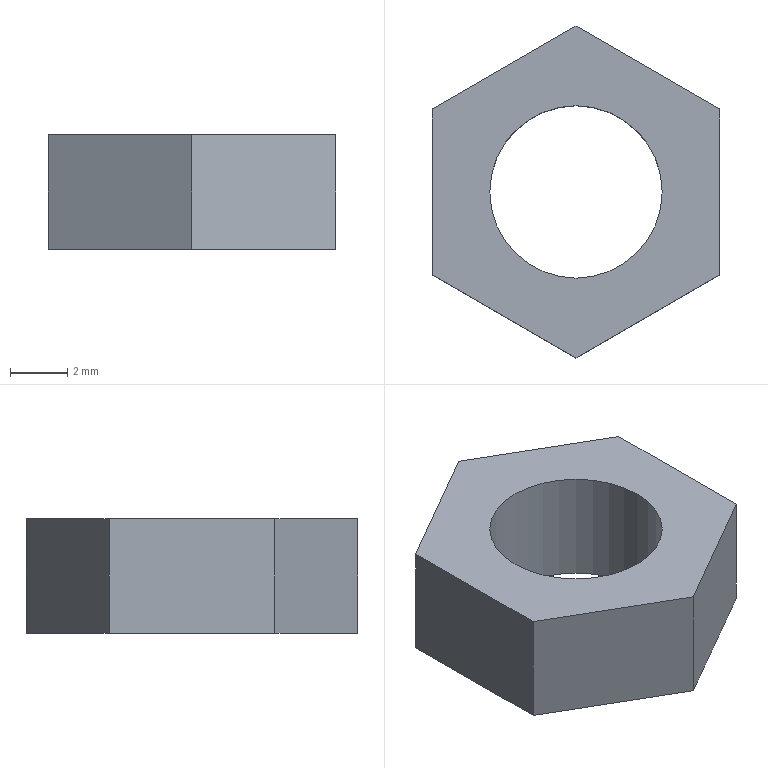Part | STEP file | M6 nut | 1 solid | 10 faces | box 10 x 11.547 x 4 mm | volume 233.313 mm3 | plane 8 | cylinder 2 | commonest cylinder face diameters 6 x2
STEP:
#1=CARTESIAN_POINT('',(0.,0.,0.));
#2=DIRECTION('',(0.,0.,1.));
#3=DIRECTION('',(1.,0.,0.));
#4=AXIS2_PLACEMENT_3D('',#1,#2,#3);
#5=CARTESIAN_POINT('',(-3.,0.,4.));
#6=VERTEX_POINT('',#5);
#7=CARTESIAN_POINT('',(-3.,0.,0.));
#8=VERTEX_POINT('',#7);
#9=CARTESIAN_POINT('',(-3.,0.,4.));
#10=DIRECTION('',(0.,0.,-1.));
#11=VECTOR('',#10,1.);
#12=LINE('',#9,#11);
#13=CARTESIAN_POINT('',(0.,0.,4.));
#14=DIRECTION('',(0.,0.,-1.));
#15=DIRECTION('',(-1.,0.,0.));
#16=AXIS2_PLACEMENT_3D('',#13,#14,#15);
#17=CYLINDRICAL_SURFACE('',#16,3.);
#18=CARTESIAN_POINT('',(6.283,0.));
#19=DIRECTION('',(0.,1.));
#20=VECTOR('',#19,1.);
#21=LINE('',#18,#20);
#22=(GEOMETRIC_REPRESENTATION_CONTEXT(2)PARAMETRIC_REPRESENTATION_CONTEXT()REPRESENTATION_CONTEXT('',''));
#23=DEFINITIONAL_REPRESENTATION('',(#21),#22);
#24=PCURVE('',#17,#23);
#25=CARTESIAN_POINT('',(0.,0.,4.));
#26=DIRECTION('',(0.,0.,-1.));
#27=DIRECTION('',(-1.,0.,0.));
#28=AXIS2_PLACEMENT_3D('',#25,#26,#27);
#29=CYLINDRICAL_SURFACE('',#28,3.);
#30=CARTESIAN_POINT('',(0.,0.));
#31=DIRECTION('',(0.,1.));
#32=VECTOR('',#31,1.);
#33=LINE('',#30,#32);
#34=(GEOMETRIC_REPRESENTATION_CONTEXT(2)PARAMETRIC_REPRESENTATION_CONTEXT()REPRESENTATION_CONTEXT('',''));
#35=DEFINITIONAL_REPRESENTATION('',(#33),#34);
#36=PCURVE('',#29,#35);
#37=SURFACE_CURVE('',#12,(#24,#36),.PCURVE_S1.);
#38=EDGE_CURVE('',#6,#8,#37,.T.);
#39=ORIENTED_EDGE('',*,*,#38,.T.);
#40=CARTESIAN_POINT('',(3.,0.,0.));
#41=VERTEX_POINT('',#40);
#42=CARTESIAN_POINT('',(0.,0.,0.));
#43=DIRECTION('',(0.,0.,1.));
#44=DIRECTION('',(1.,0.,0.));
#45=AXIS2_PLACEMENT_3D('',#42,#43,#44);
#46=CIRCLE('',#45,3.);
#47=CARTESIAN_POINT('',(9.425,4.));
#48=DIRECTION('',(-1.,0.));
#49=VECTOR('',#48,1.);
#50=LINE('',#47,#49);
#51=(GEOMETRIC_REPRESENTATION_CONTEXT(2)PARAMETRIC_REPRESENTATION_CONTEXT()REPRESENTATION_CONTEXT('',''));
#52=DEFINITIONAL_REPRESENTATION('',(#50),#51);
#53=PCURVE('',#17,#52);
#54=CARTESIAN_POINT('',(0.,0.,0.));
#55=DIRECTION('',(0.,0.,1.));
#56=DIRECTION('',(1.,0.,0.));
#57=AXIS2_PLACEMENT_3D('',#54,#55,#56);
#58=PLANE('',#57);
#59=CARTESIAN_POINT('',(0.,0.));
#60=DIRECTION('',(1.,0.));
#61=AXIS2_PLACEMENT_2D('',#59,#60);
#62=CIRCLE('',#61,3.);
#63=(GEOMETRIC_REPRESENTATION_CONTEXT(2)PARAMETRIC_REPRESENTATION_CONTEXT()REPRESENTATION_CONTEXT('',''));
#64=DEFINITIONAL_REPRESENTATION('',(#62),#63);
#65=PCURVE('',#58,#64);
#66=SURFACE_CURVE('',#46,(#53,#65),.PCURVE_S1.);
#67=EDGE_CURVE('',#8,#41,#66,.T.);
#68=ORIENTED_EDGE('',*,*,#67,.T.);
#69=CARTESIAN_POINT('',(3.,0.,4.));
#70=VERTEX_POINT('',#69);
#71=CARTESIAN_POINT('',(3.,0.,4.));
#72=DIRECTION('',(0.,0.,-1.));
#73=VECTOR('',#72,1.);
#74=LINE('',#71,#73);
#75=CARTESIAN_POINT('',(3.142,0.));
#76=DIRECTION('',(0.,1.));
#77=VECTOR('',#76,1.);
#78=LINE('',#75,#77);
#79=(GEOMETRIC_REPRESENTATION_CONTEXT(2)PARAMETRIC_REPRESENTATION_CONTEXT()REPRESENTATION_CONTEXT('',''));
#80=DEFINITIONAL_REPRESENTATION('',(#78),#79);
#81=PCURVE('',#17,#80);
#82=CARTESIAN_POINT('',(3.142,0.));
#83=DIRECTION('',(0.,1.));
#84=VECTOR('',#83,1.);
#85=LINE('',#82,#84);
#86=(GEOMETRIC_REPRESENTATION_CONTEXT(2)PARAMETRIC_REPRESENTATION_CONTEXT()REPRESENTATION_CONTEXT('',''));
#87=DEFINITIONAL_REPRESENTATION('',(#85),#86);
#88=PCURVE('',#29,#87);
#89=SURFACE_CURVE('',#74,(#81,#88),.PCURVE_S1.);
#90=EDGE_CURVE('',#70,#41,#89,.T.);
#91=ORIENTED_EDGE('',*,*,#90,.F.);
#92=CARTESIAN_POINT('',(0.,0.,4.));
#93=DIRECTION('',(0.,0.,1.));
#94=DIRECTION('',(1.,0.,0.));
#95=AXIS2_PLACEMENT_3D('',#92,#93,#94);
#96=CIRCLE('',#95,3.);
#97=CARTESIAN_POINT('',(9.425,0.));
#98=DIRECTION('',(-1.,0.));
#99=VECTOR('',#98,1.);
#100=LINE('',#97,#99);
#101=(GEOMETRIC_REPRESENTATION_CONTEXT(2)PARAMETRIC_REPRESENTATION_CONTEXT()REPRESENTATION_CONTEXT('',''));
#102=DEFINITIONAL_REPRESENTATION('',(#100),#101);
#103=PCURVE('',#17,#102);
#104=CARTESIAN_POINT('',(0.,0.,4.));
#105=DIRECTION('',(0.,0.,1.));
#106=DIRECTION('',(1.,0.,0.));
#107=AXIS2_PLACEMENT_3D('',#104,#105,#106);
#108=PLANE('',#107);
#109=CARTESIAN_POINT('',(0.,0.));
#110=DIRECTION('',(1.,0.));
#111=AXIS2_PLACEMENT_2D('',#109,#110);
#112=CIRCLE('',#111,3.);
#113=(GEOMETRIC_REPRESENTATION_CONTEXT(2)PARAMETRIC_REPRESENTATION_CONTEXT()REPRESENTATION_CONTEXT('',''));
#114=DEFINITIONAL_REPRESENTATION('',(#112),#113);
#115=PCURVE('',#108,#114);
#116=SURFACE_CURVE('',#96,(#103,#115),.PCURVE_S1.);
#117=EDGE_CURVE('',#6,#70,#116,.T.);
#118=ORIENTED_EDGE('',*,*,#117,.F.);
#119=EDGE_LOOP('',(#39,#68,#91,#118));
#120=FACE_BOUND('',#119,.F.);
#121=ADVANCED_FACE('',(#120),#17,.F.);
#122=CARTESIAN_POINT('',(-5.,2.887,4.));
#123=VERTEX_POINT('',#122);
#124=CARTESIAN_POINT('',(-5.,-2.887,4.));
#125=VERTEX_POINT('',#124);
#126=CARTESIAN_POINT('',(-5.,2.887,4.));
#127=DIRECTION('',(0.,-1.,0.));
#128=VECTOR('',#127,1.);
#129=LINE('',#126,#128);
#130=CARTESIAN_POINT('',(-5.,2.887));
#131=DIRECTION('',(0.,-1.));
#132=VECTOR('',#131,1.);
#133=LINE('',#130,#132);
#134=(GEOMETRIC_REPRESENTATION_CONTEXT(2)PARAMETRIC_REPRESENTATION_CONTEXT()REPRESENTATION_CONTEXT('',''));
#135=DEFINITIONAL_REPRESENTATION('',(#133),#134);
#136=PCURVE('',#108,#135);
#137=CARTESIAN_POINT('',(-5.,2.887,4.));
#138=DIRECTION('',(1.,0.,0.));
#139=DIRECTION('',(0.,1.,0.));
#140=AXIS2_PLACEMENT_3D('',#137,#138,#139);
#141=PLANE('',#140);
#142=CARTESIAN_POINT('',(0.,0.));
#143=DIRECTION('',(-1.,0.));
#144=VECTOR('',#143,1.);
#145=LINE('',#142,#144);
#146=(GEOMETRIC_REPRESENTATION_CONTEXT(2)PARAMETRIC_REPRESENTATION_CONTEXT()REPRESENTATION_CONTEXT('',''));
#147=DEFINITIONAL_REPRESENTATION('',(#145),#146);
#148=PCURVE('',#141,#147);
#149=SURFACE_CURVE('',#129,(#136,#148),.PCURVE_S1.);
#150=EDGE_CURVE('',#123,#125,#149,.T.);
#151=ORIENTED_EDGE('',*,*,#150,.T.);
#152=CARTESIAN_POINT('',(0.,-5.774,4.));
#153=VERTEX_POINT('',#152);
#154=CARTESIAN_POINT('',(-5.,-2.887,4.));
#155=DIRECTION('',(0.866,-0.5,0.));
#156=VECTOR('',#155,1.);
#157=LINE('',#154,#156);
#158=CARTESIAN_POINT('',(-5.,-2.887));
#159=DIRECTION('',(0.866,-0.5));
#160=VECTOR('',#159,1.);
#161=LINE('',#158,#160);
#162=(GEOMETRIC_REPRESENTATION_CONTEXT(2)PARAMETRIC_REPRESENTATION_CONTEXT()REPRESENTATION_CONTEXT('',''));
#163=DEFINITIONAL_REPRESENTATION('',(#161),#162);
#164=PCURVE('',#108,#163);
#165=CARTESIAN_POINT('',(-5.,-2.887,4.));
#166=DIRECTION('',(0.5,0.866,0.));
#167=DIRECTION('',(-0.866,0.5,0.));
#168=AXIS2_PLACEMENT_3D('',#165,#166,#167);
#169=PLANE('',#168);
#170=CARTESIAN_POINT('',(0.,0.));
#171=DIRECTION('',(-1.,0.));
#172=VECTOR('',#171,1.);
#173=LINE('',#170,#172);
#174=(GEOMETRIC_REPRESENTATION_CONTEXT(2)PARAMETRIC_REPRESENTATION_CONTEXT()REPRESENTATION_CONTEXT('',''));
#175=DEFINITIONAL_REPRESENTATION('',(#173),#174);
#176=PCURVE('',#169,#175);
#177=SURFACE_CURVE('',#157,(#164,#176),.PCURVE_S1.);
#178=EDGE_CURVE('',#125,#153,#177,.T.);
#179=ORIENTED_EDGE('',*,*,#178,.T.);
#180=CARTESIAN_POINT('',(5.,-2.887,4.));
#181=VERTEX_POINT('',#180);
#182=CARTESIAN_POINT('',(0.,-5.774,4.));
#183=DIRECTION('',(0.866,0.5,0.));
#184=VECTOR('',#183,1.);
#185=LINE('',#182,#184);
#186=CARTESIAN_POINT('',(0.,-5.774));
#187=DIRECTION('',(0.866,0.5));
#188=VECTOR('',#187,1.);
#189=LINE('',#186,#188);
#190=(GEOMETRIC_REPRESENTATION_CONTEXT(2)PARAMETRIC_REPRESENTATION_CONTEXT()REPRESENTATION_CONTEXT('',''));
#191=DEFINITIONAL_REPRESENTATION('',(#189),#190);
#192=PCURVE('',#108,#191);
#193=CARTESIAN_POINT('',(0.,-5.774,4.));
#194=DIRECTION('',(-0.5,0.866,0.));
#195=DIRECTION('',(-0.866,-0.5,0.));
#196=AXIS2_PLACEMENT_3D('',#193,#194,#195);
#197=PLANE('',#196);
#198=CARTESIAN_POINT('',(0.,0.));
#199=DIRECTION('',(-1.,0.));
#200=VECTOR('',#199,1.);
#201=LINE('',#198,#200);
#202=(GEOMETRIC_REPRESENTATION_CONTEXT(2)PARAMETRIC_REPRESENTATION_CONTEXT()REPRESENTATION_CONTEXT('',''));
#203=DEFINITIONAL_REPRESENTATION('',(#201),#202);
#204=PCURVE('',#197,#203);
#205=SURFACE_CURVE('',#185,(#192,#204),.PCURVE_S1.);
#206=EDGE_CURVE('',#153,#181,#205,.T.);
#207=ORIENTED_EDGE('',*,*,#206,.T.);
#208=CARTESIAN_POINT('',(5.,2.887,4.));
#209=VERTEX_POINT('',#208);
#210=CARTESIAN_POINT('',(5.,-2.887,4.));
#211=DIRECTION('',(0.,1.,0.));
#212=VECTOR('',#211,1.);
#213=LINE('',#210,#212);
#214=CARTESIAN_POINT('',(5.,-2.887));
#215=DIRECTION('',(0.,1.));
#216=VECTOR('',#215,1.);
#217=LINE('',#214,#216);
#218=(GEOMETRIC_REPRESENTATION_CONTEXT(2)PARAMETRIC_REPRESENTATION_CONTEXT()REPRESENTATION_CONTEXT('',''));
#219=DEFINITIONAL_REPRESENTATION('',(#217),#218);
#220=PCURVE('',#108,#219);
#221=CARTESIAN_POINT('',(5.,-2.887,4.));
#222=DIRECTION('',(-1.,0.,0.));
#223=DIRECTION('',(0.,0.,1.));
#224=AXIS2_PLACEMENT_3D('',#221,#222,#223);
#225=PLANE('',#224);
#226=CARTESIAN_POINT('',(0.,0.));
#227=DIRECTION('',(0.,1.));
#228=VECTOR('',#227,1.);
#229=LINE('',#226,#228);
#230=(GEOMETRIC_REPRESENTATION_CONTEXT(2)PARAMETRIC_REPRESENTATION_CONTEXT()REPRESENTATION_CONTEXT('',''));
#231=DEFINITIONAL_REPRESENTATION('',(#229),#230);
#232=PCURVE('',#225,#231);
#233=SURFACE_CURVE('',#213,(#220,#232),.PCURVE_S1.);
#234=EDGE_CURVE('',#181,#209,#233,.T.);
#235=ORIENTED_EDGE('',*,*,#234,.T.);
#236=CARTESIAN_POINT('',(0.,5.774,4.));
#237=VERTEX_POINT('',#236);
#238=CARTESIAN_POINT('',(5.,2.887,4.));
#239=DIRECTION('',(-0.866,0.5,0.));
#240=VECTOR('',#239,1.);
#241=LINE('',#238,#240);
#242=CARTESIAN_POINT('',(5.,2.887));
#243=DIRECTION('',(-0.866,0.5));
#244=VECTOR('',#243,1.);
#245=LINE('',#242,#244);
#246=(GEOMETRIC_REPRESENTATION_CONTEXT(2)PARAMETRIC_REPRESENTATION_CONTEXT()REPRESENTATION_CONTEXT('',''));
#247=DEFINITIONAL_REPRESENTATION('',(#245),#246);
#248=PCURVE('',#108,#247);
#249=CARTESIAN_POINT('',(5.,2.887,4.));
#250=DIRECTION('',(-0.5,-0.866,0.));
#251=DIRECTION('',(0.866,-0.5,0.));
#252=AXIS2_PLACEMENT_3D('',#249,#250,#251);
#253=PLANE('',#252);
#254=CARTESIAN_POINT('',(0.,0.));
#255=DIRECTION('',(-1.,0.));
#256=VECTOR('',#255,1.);
#257=LINE('',#254,#256);
#258=(GEOMETRIC_REPRESENTATION_CONTEXT(2)PARAMETRIC_REPRESENTATION_CONTEXT()REPRESENTATION_CONTEXT('',''));
#259=DEFINITIONAL_REPRESENTATION('',(#257),#258);
#260=PCURVE('',#253,#259);
#261=SURFACE_CURVE('',#241,(#248,#260),.PCURVE_S1.);
#262=EDGE_CURVE('',#209,#237,#261,.T.);
#263=ORIENTED_EDGE('',*,*,#262,.T.);
#264=CARTESIAN_POINT('',(0.,5.774,4.));
#265=DIRECTION('',(-0.866,-0.5,0.));
#266=VECTOR('',#265,1.);
#267=LINE('',#264,#266);
#268=CARTESIAN_POINT('',(0.,5.774));
#269=DIRECTION('',(-0.866,-0.5));
#270=VECTOR('',#269,1.);
#271=LINE('',#268,#270);
#272=(GEOMETRIC_REPRESENTATION_CONTEXT(2)PARAMETRIC_REPRESENTATION_CONTEXT()REPRESENTATION_CONTEXT('',''));
#273=DEFINITIONAL_REPRESENTATION('',(#271),#272);
#274=PCURVE('',#108,#273);
#275=CARTESIAN_POINT('',(0.,5.774,4.));
#276=DIRECTION('',(0.5,-0.866,0.));
#277=DIRECTION('',(0.866,0.5,0.));
#278=AXIS2_PLACEMENT_3D('',#275,#276,#277);
#279=PLANE('',#278);
#280=CARTESIAN_POINT('',(0.,0.));
#281=DIRECTION('',(-1.,0.));
#282=VECTOR('',#281,1.);
#283=LINE('',#280,#282);
#284=(GEOMETRIC_REPRESENTATION_CONTEXT(2)PARAMETRIC_REPRESENTATION_CONTEXT()REPRESENTATION_CONTEXT('',''));
#285=DEFINITIONAL_REPRESENTATION('',(#283),#284);
#286=PCURVE('',#279,#285);
#287=SURFACE_CURVE('',#267,(#274,#286),.PCURVE_S1.);
#288=EDGE_CURVE('',#237,#123,#287,.T.);
#289=ORIENTED_EDGE('',*,*,#288,.T.);
#290=EDGE_LOOP('',(#151,#179,#207,#235,#263,#289));
#291=FACE_BOUND('',#290,.T.);
#292=ORIENTED_EDGE('',*,*,#117,.F.);
#293=CARTESIAN_POINT('',(0.,0.,4.));
#294=DIRECTION('',(0.,0.,1.));
#295=DIRECTION('',(1.,0.,0.));
#296=AXIS2_PLACEMENT_3D('',#293,#294,#295);
#297=CIRCLE('',#296,3.);
#298=CARTESIAN_POINT('',(0.,0.));
#299=DIRECTION('',(1.,0.));
#300=AXIS2_PLACEMENT_2D('',#298,#299);
#301=CIRCLE('',#300,3.);
#302=(GEOMETRIC_REPRESENTATION_CONTEXT(2)PARAMETRIC_REPRESENTATION_CONTEXT()REPRESENTATION_CONTEXT('',''));
#303=DEFINITIONAL_REPRESENTATION('',(#301),#302);
#304=PCURVE('',#108,#303);
#305=CARTESIAN_POINT('',(3.142,0.));
#306=DIRECTION('',(-1.,0.));
#307=VECTOR('',#306,1.);
#308=LINE('',#305,#307);
#309=(GEOMETRIC_REPRESENTATION_CONTEXT(2)PARAMETRIC_REPRESENTATION_CONTEXT()REPRESENTATION_CONTEXT('',''));
#310=DEFINITIONAL_REPRESENTATION('',(#308),#309);
#311=PCURVE('',#29,#310);
#312=SURFACE_CURVE('',#297,(#304,#311),.PCURVE_S1.);
#313=EDGE_CURVE('',#70,#6,#312,.T.);
#314=ORIENTED_EDGE('',*,*,#313,.F.);
#315=EDGE_LOOP('',(#292,#314));
#316=FACE_BOUND('',#315,.T.);
#317=ADVANCED_FACE('',(#291,#316),#108,.T.);
#318=CARTESIAN_POINT('',(-5.,2.887,0.));
#319=VERTEX_POINT('',#318);
#320=CARTESIAN_POINT('',(-5.,-2.887,0.));
#321=VERTEX_POINT('',#320);
#322=CARTESIAN_POINT('',(-5.,2.887,0.));
#323=DIRECTION('',(0.,-1.,0.));
#324=VECTOR('',#323,1.);
#325=LINE('',#322,#324);
#326=CARTESIAN_POINT('',(-5.,2.887));
#327=DIRECTION('',(0.,-1.));
#328=VECTOR('',#327,1.);
#329=LINE('',#326,#328);
#330=(GEOMETRIC_REPRESENTATION_CONTEXT(2)PARAMETRIC_REPRESENTATION_CONTEXT()REPRESENTATION_CONTEXT('',''));
#331=DEFINITIONAL_REPRESENTATION('',(#329),#330);
#332=PCURVE('',#58,#331);
#333=CARTESIAN_POINT('',(0.,-4.));
#334=DIRECTION('',(-1.,0.));
#335=VECTOR('',#334,1.);
#336=LINE('',#333,#335);
#337=(GEOMETRIC_REPRESENTATION_CONTEXT(2)PARAMETRIC_REPRESENTATION_CONTEXT()REPRESENTATION_CONTEXT('',''));
#338=DEFINITIONAL_REPRESENTATION('',(#336),#337);
#339=PCURVE('',#141,#338);
#340=SURFACE_CURVE('',#325,(#332,#339),.PCURVE_S1.);
#341=EDGE_CURVE('',#319,#321,#340,.T.);
#342=ORIENTED_EDGE('',*,*,#341,.F.);
#343=CARTESIAN_POINT('',(0.,5.774,0.));
#344=VERTEX_POINT('',#343);
#345=CARTESIAN_POINT('',(0.,5.774,0.));
#346=DIRECTION('',(-0.866,-0.5,0.));
#347=VECTOR('',#346,1.);
#348=LINE('',#345,#347);
#349=CARTESIAN_POINT('',(0.,5.774));
#350=DIRECTION('',(-0.866,-0.5));
#351=VECTOR('',#350,1.);
#352=LINE('',#349,#351);
#353=(GEOMETRIC_REPRESENTATION_CONTEXT(2)PARAMETRIC_REPRESENTATION_CONTEXT()REPRESENTATION_CONTEXT('',''));
#354=DEFINITIONAL_REPRESENTATION('',(#352),#353);
#355=PCURVE('',#58,#354);
#356=CARTESIAN_POINT('',(0.,-4.));
#357=DIRECTION('',(-1.,0.));
#358=VECTOR('',#357,1.);
#359=LINE('',#356,#358);
#360=(GEOMETRIC_REPRESENTATION_CONTEXT(2)PARAMETRIC_REPRESENTATION_CONTEXT()REPRESENTATION_CONTEXT('',''));
#361=DEFINITIONAL_REPRESENTATION('',(#359),#360);
#362=PCURVE('',#279,#361);
#363=SURFACE_CURVE('',#348,(#355,#362),.PCURVE_S1.);
#364=EDGE_CURVE('',#344,#319,#363,.T.);
#365=ORIENTED_EDGE('',*,*,#364,.F.);
#366=CARTESIAN_POINT('',(5.,2.887,0.));
#367=VERTEX_POINT('',#366);
#368=CARTESIAN_POINT('',(5.,2.887,0.));
#369=DIRECTION('',(-0.866,0.5,0.));
#370=VECTOR('',#369,1.);
#371=LINE('',#368,#370);
#372=CARTESIAN_POINT('',(5.,2.887));
#373=DIRECTION('',(-0.866,0.5));
#374=VECTOR('',#373,1.);
#375=LINE('',#372,#374);
#376=(GEOMETRIC_REPRESENTATION_CONTEXT(2)PARAMETRIC_REPRESENTATION_CONTEXT()REPRESENTATION_CONTEXT('',''));
#377=DEFINITIONAL_REPRESENTATION('',(#375),#376);
#378=PCURVE('',#58,#377);
#379=CARTESIAN_POINT('',(0.,-4.));
#380=DIRECTION('',(-1.,0.));
#381=VECTOR('',#380,1.);
#382=LINE('',#379,#381);
#383=(GEOMETRIC_REPRESENTATION_CONTEXT(2)PARAMETRIC_REPRESENTATION_CONTEXT()REPRESENTATION_CONTEXT('',''));
#384=DEFINITIONAL_REPRESENTATION('',(#382),#383);
#385=PCURVE('',#253,#384);
#386=SURFACE_CURVE('',#371,(#378,#385),.PCURVE_S1.);
#387=EDGE_CURVE('',#367,#344,#386,.T.);
#388=ORIENTED_EDGE('',*,*,#387,.F.);
#389=CARTESIAN_POINT('',(5.,-2.887,0.));
#390=VERTEX_POINT('',#389);
#391=CARTESIAN_POINT('',(5.,-2.887,0.));
#392=DIRECTION('',(0.,1.,0.));
#393=VECTOR('',#392,1.);
#394=LINE('',#391,#393);
#395=CARTESIAN_POINT('',(5.,-2.887));
#396=DIRECTION('',(0.,1.));
#397=VECTOR('',#396,1.);
#398=LINE('',#395,#397);
#399=(GEOMETRIC_REPRESENTATION_CONTEXT(2)PARAMETRIC_REPRESENTATION_CONTEXT()REPRESENTATION_CONTEXT('',''));
#400=DEFINITIONAL_REPRESENTATION('',(#398),#399);
#401=PCURVE('',#58,#400);
#402=CARTESIAN_POINT('',(-4.,0.));
#403=DIRECTION('',(0.,1.));
#404=VECTOR('',#403,1.);
#405=LINE('',#402,#404);
#406=(GEOMETRIC_REPRESENTATION_CONTEXT(2)PARAMETRIC_REPRESENTATION_CONTEXT()REPRESENTATION_CONTEXT('',''));
#407=DEFINITIONAL_REPRESENTATION('',(#405),#406);
#408=PCURVE('',#225,#407);
#409=SURFACE_CURVE('',#394,(#401,#408),.PCURVE_S1.);
#410=EDGE_CURVE('',#390,#367,#409,.T.);
#411=ORIENTED_EDGE('',*,*,#410,.F.);
#412=CARTESIAN_POINT('',(0.,-5.774,0.));
#413=VERTEX_POINT('',#412);
#414=CARTESIAN_POINT('',(0.,-5.774,0.));
#415=DIRECTION('',(0.866,0.5,0.));
#416=VECTOR('',#415,1.);
#417=LINE('',#414,#416);
#418=CARTESIAN_POINT('',(0.,-5.774));
#419=DIRECTION('',(0.866,0.5));
#420=VECTOR('',#419,1.);
#421=LINE('',#418,#420);
#422=(GEOMETRIC_REPRESENTATION_CONTEXT(2)PARAMETRIC_REPRESENTATION_CONTEXT()REPRESENTATION_CONTEXT('',''));
#423=DEFINITIONAL_REPRESENTATION('',(#421),#422);
#424=PCURVE('',#58,#423);
#425=CARTESIAN_POINT('',(0.,-4.));
#426=DIRECTION('',(-1.,0.));
#427=VECTOR('',#426,1.);
#428=LINE('',#425,#427);
#429=(GEOMETRIC_REPRESENTATION_CONTEXT(2)PARAMETRIC_REPRESENTATION_CONTEXT()REPRESENTATION_CONTEXT('',''));
#430=DEFINITIONAL_REPRESENTATION('',(#428),#429);
#431=PCURVE('',#197,#430);
#432=SURFACE_CURVE('',#417,(#424,#431),.PCURVE_S1.);
#433=EDGE_CURVE('',#413,#390,#432,.T.);
#434=ORIENTED_EDGE('',*,*,#433,.F.);
#435=CARTESIAN_POINT('',(-5.,-2.887,0.));
#436=DIRECTION('',(0.866,-0.5,0.));
#437=VECTOR('',#436,1.);
#438=LINE('',#435,#437);
#439=CARTESIAN_POINT('',(-5.,-2.887));
#440=DIRECTION('',(0.866,-0.5));
#441=VECTOR('',#440,1.);
#442=LINE('',#439,#441);
#443=(GEOMETRIC_REPRESENTATION_CONTEXT(2)PARAMETRIC_REPRESENTATION_CONTEXT()REPRESENTATION_CONTEXT('',''));
#444=DEFINITIONAL_REPRESENTATION('',(#442),#443);
#445=PCURVE('',#58,#444);
#446=CARTESIAN_POINT('',(0.,-4.));
#447=DIRECTION('',(-1.,0.));
#448=VECTOR('',#447,1.);
#449=LINE('',#446,#448);
#450=(GEOMETRIC_REPRESENTATION_CONTEXT(2)PARAMETRIC_REPRESENTATION_CONTEXT()REPRESENTATION_CONTEXT('',''));
#451=DEFINITIONAL_REPRESENTATION('',(#449),#450);
#452=PCURVE('',#169,#451);
#453=SURFACE_CURVE('',#438,(#445,#452),.PCURVE_S1.);
#454=EDGE_CURVE('',#321,#413,#453,.T.);
#455=ORIENTED_EDGE('',*,*,#454,.F.);
#456=EDGE_LOOP('',(#342,#365,#388,#411,#434,#455));
#457=FACE_BOUND('',#456,.T.);
#458=ORIENTED_EDGE('',*,*,#67,.T.);
#459=CARTESIAN_POINT('',(0.,0.,0.));
#460=DIRECTION('',(0.,0.,1.));
#461=DIRECTION('',(1.,0.,0.));
#462=AXIS2_PLACEMENT_3D('',#459,#460,#461);
#463=CIRCLE('',#462,3.);
#464=CARTESIAN_POINT('',(0.,0.));
#465=DIRECTION('',(1.,0.));
#466=AXIS2_PLACEMENT_2D('',#464,#465);
#467=CIRCLE('',#466,3.);
#468=(GEOMETRIC_REPRESENTATION_CONTEXT(2)PARAMETRIC_REPRESENTATION_CONTEXT()REPRESENTATION_CONTEXT('',''));
#469=DEFINITIONAL_REPRESENTATION('',(#467),#468);
#470=PCURVE('',#58,#469);
#471=CARTESIAN_POINT('',(3.142,4.));
#472=DIRECTION('',(-1.,0.));
#473=VECTOR('',#472,1.);
#474=LINE('',#471,#473);
#475=(GEOMETRIC_REPRESENTATION_CONTEXT(2)PARAMETRIC_REPRESENTATION_CONTEXT()REPRESENTATION_CONTEXT('',''));
#476=DEFINITIONAL_REPRESENTATION('',(#474),#475);
#477=PCURVE('',#29,#476);
#478=SURFACE_CURVE('',#463,(#470,#477),.PCURVE_S1.);
#479=EDGE_CURVE('',#41,#8,#478,.T.);
#480=ORIENTED_EDGE('',*,*,#479,.T.);
#481=EDGE_LOOP('',(#458,#480));
#482=FACE_BOUND('',#481,.T.);
#483=ADVANCED_FACE('',(#457,#482),#58,.F.);
#484=ORIENTED_EDGE('',*,*,#341,.T.);
#485=CARTESIAN_POINT('',(-5.,-2.887,4.));
#486=DIRECTION('',(0.,0.,-1.));
#487=VECTOR('',#486,1.);
#488=LINE('',#485,#487);
#489=CARTESIAN_POINT('',(-5.774,0.));
#490=DIRECTION('',(0.,-1.));
#491=VECTOR('',#490,1.);
#492=LINE('',#489,#491);
#493=(GEOMETRIC_REPRESENTATION_CONTEXT(2)PARAMETRIC_REPRESENTATION_CONTEXT()REPRESENTATION_CONTEXT('',''));
#494=DEFINITIONAL_REPRESENTATION('',(#492),#493);
#495=PCURVE('',#141,#494);
#496=CARTESIAN_POINT('',(0.,0.));
#497=DIRECTION('',(0.,-1.));
#498=VECTOR('',#497,1.);
#499=LINE('',#496,#498);
#500=(GEOMETRIC_REPRESENTATION_CONTEXT(2)PARAMETRIC_REPRESENTATION_CONTEXT()REPRESENTATION_CONTEXT('',''));
#501=DEFINITIONAL_REPRESENTATION('',(#499),#500);
#502=PCURVE('',#169,#501);
#503=SURFACE_CURVE('',#488,(#495,#502),.PCURVE_S1.);
#504=EDGE_CURVE('',#125,#321,#503,.T.);
#505=ORIENTED_EDGE('',*,*,#504,.F.);
#506=ORIENTED_EDGE('',*,*,#150,.F.);
#507=CARTESIAN_POINT('',(-5.,2.887,4.));
#508=DIRECTION('',(0.,0.,-1.));
#509=VECTOR('',#508,1.);
#510=LINE('',#507,#509);
#511=CARTESIAN_POINT('',(0.,0.));
#512=DIRECTION('',(0.,-1.));
#513=VECTOR('',#512,1.);
#514=LINE('',#511,#513);
#515=(GEOMETRIC_REPRESENTATION_CONTEXT(2)PARAMETRIC_REPRESENTATION_CONTEXT()REPRESENTATION_CONTEXT('',''));
#516=DEFINITIONAL_REPRESENTATION('',(#514),#515);
#517=PCURVE('',#141,#516);
#518=CARTESIAN_POINT('',(-5.774,0.));
#519=DIRECTION('',(0.,-1.));
#520=VECTOR('',#519,1.);
#521=LINE('',#518,#520);
#522=(GEOMETRIC_REPRESENTATION_CONTEXT(2)PARAMETRIC_REPRESENTATION_CONTEXT()REPRESENTATION_CONTEXT('',''));
#523=DEFINITIONAL_REPRESENTATION('',(#521),#522);
#524=PCURVE('',#279,#523);
#525=SURFACE_CURVE('',#510,(#517,#524),.PCURVE_S1.);
#526=EDGE_CURVE('',#123,#319,#525,.T.);
#527=ORIENTED_EDGE('',*,*,#526,.T.);
#528=EDGE_LOOP('',(#484,#505,#506,#527));
#529=FACE_BOUND('',#528,.T.);
#530=ADVANCED_FACE('',(#529),#141,.F.);
#531=ORIENTED_EDGE('',*,*,#454,.T.);
#532=CARTESIAN_POINT('',(0.,-5.774,4.));
#533=DIRECTION('',(0.,0.,-1.));
#534=VECTOR('',#533,1.);
#535=LINE('',#532,#534);
#536=CARTESIAN_POINT('',(-5.774,0.));
#537=DIRECTION('',(0.,-1.));
#538=VECTOR('',#537,1.);
#539=LINE('',#536,#538);
#540=(GEOMETRIC_REPRESENTATION_CONTEXT(2)PARAMETRIC_REPRESENTATION_CONTEXT()REPRESENTATION_CONTEXT('',''));
#541=DEFINITIONAL_REPRESENTATION('',(#539),#540);
#542=PCURVE('',#169,#541);
#543=CARTESIAN_POINT('',(0.,0.));
#544=DIRECTION('',(0.,-1.));
#545=VECTOR('',#544,1.);
#546=LINE('',#543,#545);
#547=(GEOMETRIC_REPRESENTATION_CONTEXT(2)PARAMETRIC_REPRESENTATION_CONTEXT()REPRESENTATION_CONTEXT('',''));
#548=DEFINITIONAL_REPRESENTATION('',(#546),#547);
#549=PCURVE('',#197,#548);
#550=SURFACE_CURVE('',#535,(#542,#549),.PCURVE_S1.);
#551=EDGE_CURVE('',#153,#413,#550,.T.);
#552=ORIENTED_EDGE('',*,*,#551,.F.);
#553=ORIENTED_EDGE('',*,*,#178,.F.);
#554=ORIENTED_EDGE('',*,*,#504,.T.);
#555=EDGE_LOOP('',(#531,#552,#553,#554));
#556=FACE_BOUND('',#555,.T.);
#557=ADVANCED_FACE('',(#556),#169,.F.);
#558=ORIENTED_EDGE('',*,*,#433,.T.);
#559=CARTESIAN_POINT('',(5.,-2.887,4.));
#560=DIRECTION('',(0.,0.,-1.));
#561=VECTOR('',#560,1.);
#562=LINE('',#559,#561);
#563=CARTESIAN_POINT('',(-5.774,0.));
#564=DIRECTION('',(0.,-1.));
#565=VECTOR('',#564,1.);
#566=LINE('',#563,#565);
#567=(GEOMETRIC_REPRESENTATION_CONTEXT(2)PARAMETRIC_REPRESENTATION_CONTEXT()REPRESENTATION_CONTEXT('',''));
#568=DEFINITIONAL_REPRESENTATION('',(#566),#567);
#569=PCURVE('',#197,#568);
#570=CARTESIAN_POINT('',(0.,0.));
#571=DIRECTION('',(-1.,0.));
#572=VECTOR('',#571,1.);
#573=LINE('',#570,#572);
#574=(GEOMETRIC_REPRESENTATION_CONTEXT(2)PARAMETRIC_REPRESENTATION_CONTEXT()REPRESENTATION_CONTEXT('',''));
#575=DEFINITIONAL_REPRESENTATION('',(#573),#574);
#576=PCURVE('',#225,#575);
#577=SURFACE_CURVE('',#562,(#569,#576),.PCURVE_S1.);
#578=EDGE_CURVE('',#181,#390,#577,.T.);
#579=ORIENTED_EDGE('',*,*,#578,.F.);
#580=ORIENTED_EDGE('',*,*,#206,.F.);
#581=ORIENTED_EDGE('',*,*,#551,.T.);
#582=EDGE_LOOP('',(#558,#579,#580,#581));
#583=FACE_BOUND('',#582,.T.);
#584=ADVANCED_FACE('',(#583),#197,.F.);
#585=ORIENTED_EDGE('',*,*,#410,.T.);
#586=CARTESIAN_POINT('',(5.,2.887,4.));
#587=DIRECTION('',(0.,0.,-1.));
#588=VECTOR('',#587,1.);
#589=LINE('',#586,#588);
#590=CARTESIAN_POINT('',(0.,5.774));
#591=DIRECTION('',(-1.,0.));
#592=VECTOR('',#591,1.);
#593=LINE('',#590,#592);
#594=(GEOMETRIC_REPRESENTATION_CONTEXT(2)PARAMETRIC_REPRESENTATION_CONTEXT()REPRESENTATION_CONTEXT('',''));
#595=DEFINITIONAL_REPRESENTATION('',(#593),#594);
#596=PCURVE('',#225,#595);
#597=CARTESIAN_POINT('',(0.,0.));
#598=DIRECTION('',(0.,-1.));
#599=VECTOR('',#598,1.);
#600=LINE('',#597,#599);
#601=(GEOMETRIC_REPRESENTATION_CONTEXT(2)PARAMETRIC_REPRESENTATION_CONTEXT()REPRESENTATION_CONTEXT('',''));
#602=DEFINITIONAL_REPRESENTATION('',(#600),#601);
#603=PCURVE('',#253,#602);
#604=SURFACE_CURVE('',#589,(#596,#603),.PCURVE_S1.);
#605=EDGE_CURVE('',#209,#367,#604,.T.);
#606=ORIENTED_EDGE('',*,*,#605,.F.);
#607=ORIENTED_EDGE('',*,*,#234,.F.);
#608=ORIENTED_EDGE('',*,*,#578,.T.);
#609=EDGE_LOOP('',(#585,#606,#607,#608));
#610=FACE_BOUND('',#609,.T.);
#611=ADVANCED_FACE('',(#610),#225,.F.);
#612=ORIENTED_EDGE('',*,*,#387,.T.);
#613=CARTESIAN_POINT('',(0.,5.774,4.));
#614=DIRECTION('',(0.,0.,-1.));
#615=VECTOR('',#614,1.);
#616=LINE('',#613,#615);
#617=CARTESIAN_POINT('',(-5.774,0.));
#618=DIRECTION('',(0.,-1.));
#619=VECTOR('',#618,1.);
#620=LINE('',#617,#619);
#621=(GEOMETRIC_REPRESENTATION_CONTEXT(2)PARAMETRIC_REPRESENTATION_CONTEXT()REPRESENTATION_CONTEXT('',''));
#622=DEFINITIONAL_REPRESENTATION('',(#620),#621);
#623=PCURVE('',#253,#622);
#624=CARTESIAN_POINT('',(0.,0.));
#625=DIRECTION('',(0.,-1.));
#626=VECTOR('',#625,1.);
#627=LINE('',#624,#626);
#628=(GEOMETRIC_REPRESENTATION_CONTEXT(2)PARAMETRIC_REPRESENTATION_CONTEXT()REPRESENTATION_CONTEXT('',''));
#629=DEFINITIONAL_REPRESENTATION('',(#627),#628);
#630=PCURVE('',#279,#629);
#631=SURFACE_CURVE('',#616,(#623,#630),.PCURVE_S1.);
#632=EDGE_CURVE('',#237,#344,#631,.T.);
#633=ORIENTED_EDGE('',*,*,#632,.F.);
#634=ORIENTED_EDGE('',*,*,#262,.F.);
#635=ORIENTED_EDGE('',*,*,#605,.T.);
#636=EDGE_LOOP('',(#612,#633,#634,#635));
#637=FACE_BOUND('',#636,.T.);
#638=ADVANCED_FACE('',(#637),#253,.F.);
#639=ORIENTED_EDGE('',*,*,#364,.T.);
#640=ORIENTED_EDGE('',*,*,#526,.F.);
#641=ORIENTED_EDGE('',*,*,#288,.F.);
#642=ORIENTED_EDGE('',*,*,#632,.T.);
#643=EDGE_LOOP('',(#639,#640,#641,#642));
#644=FACE_BOUND('',#643,.T.);
#645=ADVANCED_FACE('',(#644),#279,.F.);
#646=ORIENTED_EDGE('',*,*,#479,.T.);
#647=ORIENTED_EDGE('',*,*,#38,.F.);
#648=ORIENTED_EDGE('',*,*,#313,.F.);
#649=ORIENTED_EDGE('',*,*,#90,.T.);
#650=EDGE_LOOP('',(#646,#647,#648,#649));
#651=FACE_BOUND('',#650,.F.);
#652=ADVANCED_FACE('',(#651),#29,.F.);
#653=CLOSED_SHELL('',(#121,#317,#483,#530,#557,#584,#611,#638,#645,#652));
#654=MANIFOLD_SOLID_BREP('',#653);
#655=(LENGTH_UNIT()NAMED_UNIT(*)SI_UNIT(.MILLI.,.METRE.));
#656=UNCERTAINTY_MEASURE_WITH_UNIT(LENGTH_MEASURE(0.0000001),#655,'','');
#657=(NAMED_UNIT(*)PLANE_ANGLE_UNIT()SI_UNIT($,.RADIAN.));
#658=(NAMED_UNIT(*)SI_UNIT($,.STERADIAN.)SOLID_ANGLE_UNIT());
#659=(GEOMETRIC_REPRESENTATION_CONTEXT(3)GLOBAL_UNCERTAINTY_ASSIGNED_CONTEXT((#656))GLOBAL_UNIT_ASSIGNED_CONTEXT((#655,#657,#658))REPRESENTATION_CONTEXT('',''));
#660=ADVANCED_BREP_SHAPE_REPRESENTATION('',(#4,#654),#659);